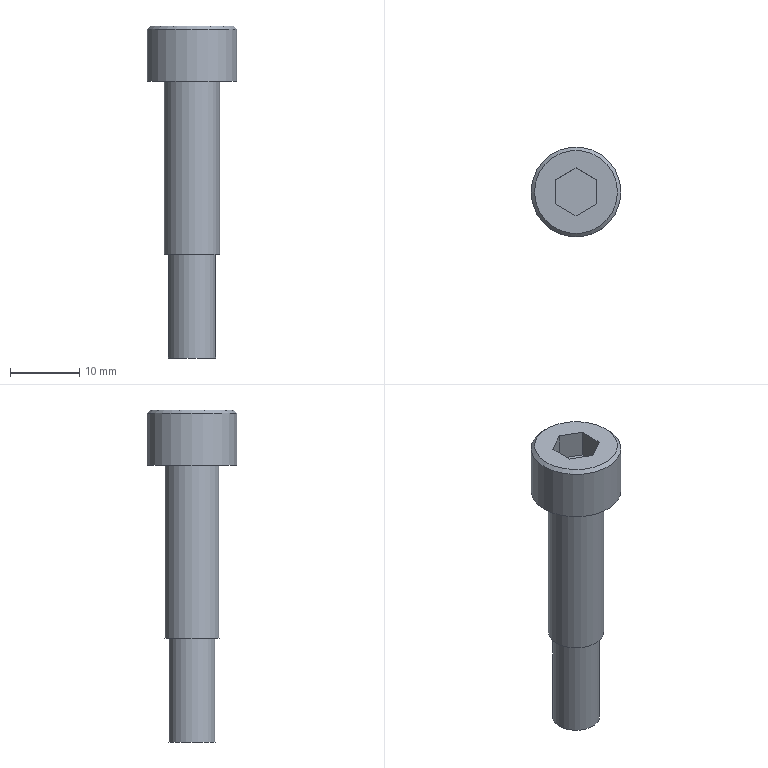Part | STEP file | M3-10_id154_x_t | 1 solid | 15 faces | box 13 x 13 x 48 mm | volume 2734 mm3 | plane 11 | cylinder 3 | cone 1 | commonest cylinder face diameters 6.8 x1 8 x1 13 x1
STEP:
#1=CARTESIAN_POINT('',(-180.986,-124.,-47.));
#2=VERTEX_POINT('',#1);
#3=CARTESIAN_POINT('',(-177.586,-124.,-47.));
#4=DIRECTION('',(0.,0.,-1.));
#5=DIRECTION('',(-1.,0.,0.));
#6=AXIS2_PLACEMENT_3D('',#3,#4,#5);
#7=CIRCLE('',#6,3.4);
#8=EDGE_CURVE('',#2,#2,#7,.T.);
#9=ORIENTED_EDGE('',*,*,#8,.F.);
#10=EDGE_LOOP('',(#9));
#11=FACE_BOUND('',#10,.T.);
#12=CARTESIAN_POINT('',(-173.586,-124.,-47.));
#13=VERTEX_POINT('',#12);
#14=CARTESIAN_POINT('',(-177.586,-124.,-47.));
#15=DIRECTION('',(0.,0.,1.));
#16=DIRECTION('',(1.,0.,0.));
#17=AXIS2_PLACEMENT_3D('',#14,#15,#16);
#18=CIRCLE('',#17,4.);
#19=EDGE_CURVE('',#13,#13,#18,.T.);
#20=ORIENTED_EDGE('',*,*,#19,.F.);
#21=EDGE_LOOP('',(#20));
#22=FACE_BOUND('',#21,.T.);
#23=CARTESIAN_POINT('',(-177.586,-124.,-47.));
#24=DIRECTION('',(0.,0.,-1.));
#25=DIRECTION('',(-1.,0.,0.));
#26=AXIS2_PLACEMENT_3D('',#23,#24,#25);
#27=PLANE('',#26);
#28=ADVANCED_FACE('',(#11,#22),#27,.T.);
#29=CARTESIAN_POINT('',(-181.586,-124.,-22.));
#30=VERTEX_POINT('',#29);
#31=CARTESIAN_POINT('',(-177.586,-124.,-22.));
#32=DIRECTION('',(0.,0.,1.));
#33=DIRECTION('',(-1.,0.,0.));
#34=AXIS2_PLACEMENT_3D('',#31,#32,#33);
#35=CIRCLE('',#34,4.);
#36=EDGE_CURVE('',#30,#30,#35,.T.);
#37=ORIENTED_EDGE('',*,*,#36,.F.);
#38=EDGE_LOOP('',(#37));
#39=FACE_BOUND('',#38,.T.);
#40=ORIENTED_EDGE('',*,*,#19,.T.);
#41=EDGE_LOOP('',(#40));
#42=FACE_BOUND('',#41,.T.);
#43=CARTESIAN_POINT('',(-177.586,-124.,-47.));
#44=DIRECTION('',(0.,0.,1.));
#45=DIRECTION('',(1.,0.,0.));
#46=AXIS2_PLACEMENT_3D('',#43,#44,#45);
#47=CYLINDRICAL_SURFACE('',#46,4.);
#48=ADVANCED_FACE('',(#39,#42),#47,.T.);
#49=CARTESIAN_POINT('',(-174.186,-124.,-62.));
#50=VERTEX_POINT('',#49);
#51=CARTESIAN_POINT('',(-177.586,-124.,-62.));
#52=DIRECTION('',(0.,0.,1.));
#53=DIRECTION('',(1.,0.,0.));
#54=AXIS2_PLACEMENT_3D('',#51,#52,#53);
#55=CIRCLE('',#54,3.4);
#56=EDGE_CURVE('',#50,#50,#55,.T.);
#57=ORIENTED_EDGE('',*,*,#56,.F.);
#58=EDGE_LOOP('',(#57));
#59=FACE_OUTER_BOUND('',#58,.T.);
#60=CARTESIAN_POINT('',(-177.586,-124.,-62.));
#61=DIRECTION('',(0.,0.,-1.));
#62=DIRECTION('',(-1.,0.,0.));
#63=AXIS2_PLACEMENT_3D('',#60,#61,#62);
#64=PLANE('',#63);
#65=ADVANCED_FACE('',(#59),#64,.T.);
#66=ORIENTED_EDGE('',*,*,#56,.T.);
#67=EDGE_LOOP('',(#66));
#68=FACE_BOUND('',#67,.T.);
#69=ORIENTED_EDGE('',*,*,#8,.T.);
#70=EDGE_LOOP('',(#69));
#71=FACE_BOUND('',#70,.T.);
#72=CARTESIAN_POINT('',(-177.586,-124.,-47.));
#73=DIRECTION('',(0.,0.,-1.));
#74=DIRECTION('',(1.,0.,0.));
#75=AXIS2_PLACEMENT_3D('',#72,#73,#74);
#76=CYLINDRICAL_SURFACE('',#75,3.4);
#77=ADVANCED_FACE('',(#68,#71),#76,.T.);
#78=CARTESIAN_POINT('',(-180.586,-122.268,-14.));
#79=VERTEX_POINT('',#78);
#80=CARTESIAN_POINT('',(-180.586,-125.732,-14.));
#81=VERTEX_POINT('',#80);
#82=CARTESIAN_POINT('',(-180.586,-122.268,-14.));
#83=DIRECTION('',(0.,-1.,0.));
#84=VECTOR('',#83,1.);
#85=LINE('',#82,#84);
#86=EDGE_CURVE('',#79,#81,#85,.T.);
#87=ORIENTED_EDGE('',*,*,#86,.F.);
#88=CARTESIAN_POINT('',(-177.586,-120.536,-14.));
#89=VERTEX_POINT('',#88);
#90=CARTESIAN_POINT('',(-177.586,-120.536,-14.));
#91=DIRECTION('',(-0.866,-0.5,0.));
#92=VECTOR('',#91,1.);
#93=LINE('',#90,#92);
#94=EDGE_CURVE('',#89,#79,#93,.T.);
#95=ORIENTED_EDGE('',*,*,#94,.F.);
#96=CARTESIAN_POINT('',(-174.586,-122.268,-14.));
#97=VERTEX_POINT('',#96);
#98=CARTESIAN_POINT('',(-174.586,-122.268,-14.));
#99=DIRECTION('',(-0.866,0.5,0.));
#100=VECTOR('',#99,1.);
#101=LINE('',#98,#100);
#102=EDGE_CURVE('',#97,#89,#101,.T.);
#103=ORIENTED_EDGE('',*,*,#102,.F.);
#104=CARTESIAN_POINT('',(-174.586,-125.732,-14.));
#105=VERTEX_POINT('',#104);
#106=CARTESIAN_POINT('',(-174.586,-125.732,-14.));
#107=DIRECTION('',(0.,1.,0.));
#108=VECTOR('',#107,1.);
#109=LINE('',#106,#108);
#110=EDGE_CURVE('',#105,#97,#109,.T.);
#111=ORIENTED_EDGE('',*,*,#110,.F.);
#112=CARTESIAN_POINT('',(-177.586,-127.464,-14.));
#113=VERTEX_POINT('',#112);
#114=CARTESIAN_POINT('',(-177.586,-127.464,-14.));
#115=DIRECTION('',(0.866,0.5,0.));
#116=VECTOR('',#115,1.);
#117=LINE('',#114,#116);
#118=EDGE_CURVE('',#113,#105,#117,.T.);
#119=ORIENTED_EDGE('',*,*,#118,.F.);
#120=CARTESIAN_POINT('',(-180.586,-125.732,-14.));
#121=DIRECTION('',(0.866,-0.5,0.));
#122=VECTOR('',#121,1.);
#123=LINE('',#120,#122);
#124=EDGE_CURVE('',#81,#113,#123,.T.);
#125=ORIENTED_EDGE('',*,*,#124,.F.);
#126=EDGE_LOOP('',(#87,#95,#103,#111,#119,#125));
#127=FACE_BOUND('',#126,.T.);
#128=CARTESIAN_POINT('',(-171.586,-124.,-14.));
#129=VERTEX_POINT('',#128);
#130=CARTESIAN_POINT('',(-177.586,-124.,-14.));
#131=DIRECTION('',(0.,0.,1.));
#132=DIRECTION('',(1.,0.,0.));
#133=AXIS2_PLACEMENT_3D('',#130,#131,#132);
#134=CIRCLE('',#133,6.);
#135=EDGE_CURVE('',#129,#129,#134,.T.);
#136=ORIENTED_EDGE('',*,*,#135,.T.);
#137=EDGE_LOOP('',(#136));
#138=FACE_BOUND('',#137,.T.);
#139=CARTESIAN_POINT('',(-177.586,-124.,-14.));
#140=DIRECTION('',(0.,0.,1.));
#141=DIRECTION('',(1.,0.,0.));
#142=AXIS2_PLACEMENT_3D('',#139,#140,#141);
#143=PLANE('',#142);
#144=ADVANCED_FACE('',(#127,#138),#143,.T.);
#145=ORIENTED_EDGE('',*,*,#36,.T.);
#146=EDGE_LOOP('',(#145));
#147=FACE_BOUND('',#146,.T.);
#148=CARTESIAN_POINT('',(-171.086,-124.,-22.));
#149=VERTEX_POINT('',#148);
#150=CARTESIAN_POINT('',(-177.586,-124.,-22.));
#151=DIRECTION('',(0.,0.,1.));
#152=DIRECTION('',(1.,0.,0.));
#153=AXIS2_PLACEMENT_3D('',#150,#151,#152);
#154=CIRCLE('',#153,6.5);
#155=EDGE_CURVE('',#149,#149,#154,.T.);
#156=ORIENTED_EDGE('',*,*,#155,.F.);
#157=EDGE_LOOP('',(#156));
#158=FACE_BOUND('',#157,.T.);
#159=CARTESIAN_POINT('',(-177.586,-124.,-22.));
#160=DIRECTION('',(0.,0.,-1.));
#161=DIRECTION('',(-1.,0.,0.));
#162=AXIS2_PLACEMENT_3D('',#159,#160,#161);
#163=PLANE('',#162);
#164=ADVANCED_FACE('',(#147,#158),#163,.T.);
#165=CARTESIAN_POINT('',(-171.086,-124.,-14.5));
#166=VERTEX_POINT('',#165);
#167=CARTESIAN_POINT('',(-177.586,-124.,-14.5));
#168=DIRECTION('',(0.,0.,-1.));
#169=DIRECTION('',(1.,0.,0.));
#170=AXIS2_PLACEMENT_3D('',#167,#168,#169);
#171=CIRCLE('',#170,6.5);
#172=EDGE_CURVE('',#166,#166,#171,.T.);
#173=ORIENTED_EDGE('',*,*,#172,.T.);
#174=EDGE_LOOP('',(#173));
#175=FACE_BOUND('',#174,.T.);
#176=ORIENTED_EDGE('',*,*,#155,.T.);
#177=EDGE_LOOP('',(#176));
#178=FACE_BOUND('',#177,.T.);
#179=CARTESIAN_POINT('',(-177.586,-124.,-22.));
#180=DIRECTION('',(0.,0.,1.));
#181=DIRECTION('',(1.,0.,0.));
#182=AXIS2_PLACEMENT_3D('',#179,#180,#181);
#183=CYLINDRICAL_SURFACE('',#182,6.5);
#184=ADVANCED_FACE('',(#175,#178),#183,.T.);
#185=ORIENTED_EDGE('',*,*,#135,.F.);
#186=EDGE_LOOP('',(#185));
#187=FACE_BOUND('',#186,.T.);
#188=ORIENTED_EDGE('',*,*,#172,.F.);
#189=EDGE_LOOP('',(#188));
#190=FACE_BOUND('',#189,.T.);
#191=CARTESIAN_POINT('',(-177.586,-124.,-14.5));
#192=DIRECTION('',(0.,0.,-1.));
#193=DIRECTION('',(-1.,0.,0.));
#194=AXIS2_PLACEMENT_3D('',#191,#192,#193);
#195=CONICAL_SURFACE('',#194,6.5,45.);
#196=ADVANCED_FACE('',(#187,#190),#195,.T.);
#197=ORIENTED_EDGE('',*,*,#86,.T.);
#198=CARTESIAN_POINT('',(-180.586,-125.732,-18.));
#199=VERTEX_POINT('',#198);
#200=CARTESIAN_POINT('',(-180.586,-125.732,-18.));
#201=DIRECTION('',(0.,0.,-1.));
#202=VECTOR('',#201,1.);
#203=LINE('',#200,#202);
#204=EDGE_CURVE('',#81,#199,#203,.T.);
#205=ORIENTED_EDGE('',*,*,#204,.T.);
#206=CARTESIAN_POINT('',(-180.586,-122.268,-18.));
#207=VERTEX_POINT('',#206);
#208=CARTESIAN_POINT('',(-180.586,-122.268,-18.));
#209=DIRECTION('',(0.,1.,0.));
#210=VECTOR('',#209,1.);
#211=LINE('',#208,#210);
#212=EDGE_CURVE('',#199,#207,#211,.T.);
#213=ORIENTED_EDGE('',*,*,#212,.T.);
#214=CARTESIAN_POINT('',(-180.586,-122.268,-18.));
#215=DIRECTION('',(0.,0.,-1.));
#216=VECTOR('',#215,1.);
#217=LINE('',#214,#216);
#218=EDGE_CURVE('',#79,#207,#217,.T.);
#219=ORIENTED_EDGE('',*,*,#218,.F.);
#220=EDGE_LOOP('',(#197,#205,#213,#219));
#221=FACE_OUTER_BOUND('',#220,.T.);
#222=CARTESIAN_POINT('',(-180.586,-122.268,-18.));
#223=DIRECTION('',(-1.,0.,0.));
#224=DIRECTION('',(0.,-1.,0.));
#225=AXIS2_PLACEMENT_3D('',#222,#223,#224);
#226=PLANE('',#225);
#227=ADVANCED_FACE('',(#221),#226,.F.);
#228=ORIENTED_EDGE('',*,*,#124,.T.);
#229=CARTESIAN_POINT('',(-177.586,-127.464,-18.));
#230=VERTEX_POINT('',#229);
#231=CARTESIAN_POINT('',(-177.586,-127.464,-18.));
#232=DIRECTION('',(0.,0.,-1.));
#233=VECTOR('',#232,1.);
#234=LINE('',#231,#233);
#235=EDGE_CURVE('',#113,#230,#234,.T.);
#236=ORIENTED_EDGE('',*,*,#235,.T.);
#237=CARTESIAN_POINT('',(-180.586,-125.732,-18.));
#238=DIRECTION('',(-0.866,0.5,0.));
#239=VECTOR('',#238,1.);
#240=LINE('',#237,#239);
#241=EDGE_CURVE('',#230,#199,#240,.T.);
#242=ORIENTED_EDGE('',*,*,#241,.T.);
#243=ORIENTED_EDGE('',*,*,#204,.F.);
#244=EDGE_LOOP('',(#228,#236,#242,#243));
#245=FACE_OUTER_BOUND('',#244,.T.);
#246=CARTESIAN_POINT('',(-180.586,-125.732,-18.));
#247=DIRECTION('',(-0.5,-0.866,0.));
#248=DIRECTION('',(0.866,-0.5,0.));
#249=AXIS2_PLACEMENT_3D('',#246,#247,#248);
#250=PLANE('',#249);
#251=ADVANCED_FACE('',(#245),#250,.F.);
#252=ORIENTED_EDGE('',*,*,#118,.T.);
#253=CARTESIAN_POINT('',(-174.586,-125.732,-18.));
#254=VERTEX_POINT('',#253);
#255=CARTESIAN_POINT('',(-174.586,-125.732,-18.));
#256=DIRECTION('',(0.,0.,-1.));
#257=VECTOR('',#256,1.);
#258=LINE('',#255,#257);
#259=EDGE_CURVE('',#105,#254,#258,.T.);
#260=ORIENTED_EDGE('',*,*,#259,.T.);
#261=CARTESIAN_POINT('',(-177.586,-127.464,-18.));
#262=DIRECTION('',(-0.866,-0.5,0.));
#263=VECTOR('',#262,1.);
#264=LINE('',#261,#263);
#265=EDGE_CURVE('',#254,#230,#264,.T.);
#266=ORIENTED_EDGE('',*,*,#265,.T.);
#267=ORIENTED_EDGE('',*,*,#235,.F.);
#268=EDGE_LOOP('',(#252,#260,#266,#267));
#269=FACE_OUTER_BOUND('',#268,.T.);
#270=CARTESIAN_POINT('',(-177.586,-127.464,-18.));
#271=DIRECTION('',(0.5,-0.866,0.));
#272=DIRECTION('',(0.866,0.5,0.));
#273=AXIS2_PLACEMENT_3D('',#270,#271,#272);
#274=PLANE('',#273);
#275=ADVANCED_FACE('',(#269),#274,.F.);
#276=ORIENTED_EDGE('',*,*,#110,.T.);
#277=CARTESIAN_POINT('',(-174.586,-122.268,-18.));
#278=VERTEX_POINT('',#277);
#279=CARTESIAN_POINT('',(-174.586,-122.268,-18.));
#280=DIRECTION('',(0.,0.,-1.));
#281=VECTOR('',#280,1.);
#282=LINE('',#279,#281);
#283=EDGE_CURVE('',#97,#278,#282,.T.);
#284=ORIENTED_EDGE('',*,*,#283,.T.);
#285=CARTESIAN_POINT('',(-174.586,-125.732,-18.));
#286=DIRECTION('',(0.,-1.,0.));
#287=VECTOR('',#286,1.);
#288=LINE('',#285,#287);
#289=EDGE_CURVE('',#278,#254,#288,.T.);
#290=ORIENTED_EDGE('',*,*,#289,.T.);
#291=ORIENTED_EDGE('',*,*,#259,.F.);
#292=EDGE_LOOP('',(#276,#284,#290,#291));
#293=FACE_OUTER_BOUND('',#292,.T.);
#294=CARTESIAN_POINT('',(-174.586,-125.732,-18.));
#295=DIRECTION('',(1.,0.,0.));
#296=DIRECTION('',(0.,1.,0.));
#297=AXIS2_PLACEMENT_3D('',#294,#295,#296);
#298=PLANE('',#297);
#299=ADVANCED_FACE('',(#293),#298,.F.);
#300=ORIENTED_EDGE('',*,*,#102,.T.);
#301=CARTESIAN_POINT('',(-177.586,-120.536,-18.));
#302=VERTEX_POINT('',#301);
#303=CARTESIAN_POINT('',(-177.586,-120.536,-18.));
#304=DIRECTION('',(0.,0.,-1.));
#305=VECTOR('',#304,1.);
#306=LINE('',#303,#305);
#307=EDGE_CURVE('',#89,#302,#306,.T.);
#308=ORIENTED_EDGE('',*,*,#307,.T.);
#309=CARTESIAN_POINT('',(-174.586,-122.268,-18.));
#310=DIRECTION('',(0.866,-0.5,0.));
#311=VECTOR('',#310,1.);
#312=LINE('',#309,#311);
#313=EDGE_CURVE('',#302,#278,#312,.T.);
#314=ORIENTED_EDGE('',*,*,#313,.T.);
#315=ORIENTED_EDGE('',*,*,#283,.F.);
#316=EDGE_LOOP('',(#300,#308,#314,#315));
#317=FACE_OUTER_BOUND('',#316,.T.);
#318=CARTESIAN_POINT('',(-174.586,-122.268,-18.));
#319=DIRECTION('',(0.5,0.866,0.));
#320=DIRECTION('',(-0.866,0.5,0.));
#321=AXIS2_PLACEMENT_3D('',#318,#319,#320);
#322=PLANE('',#321);
#323=ADVANCED_FACE('',(#317),#322,.F.);
#324=ORIENTED_EDGE('',*,*,#94,.T.);
#325=ORIENTED_EDGE('',*,*,#218,.T.);
#326=CARTESIAN_POINT('',(-177.586,-120.536,-18.));
#327=DIRECTION('',(0.866,0.5,0.));
#328=VECTOR('',#327,1.);
#329=LINE('',#326,#328);
#330=EDGE_CURVE('',#207,#302,#329,.T.);
#331=ORIENTED_EDGE('',*,*,#330,.T.);
#332=ORIENTED_EDGE('',*,*,#307,.F.);
#333=EDGE_LOOP('',(#324,#325,#331,#332));
#334=FACE_OUTER_BOUND('',#333,.T.);
#335=CARTESIAN_POINT('',(-177.586,-120.536,-18.));
#336=DIRECTION('',(-0.5,0.866,0.));
#337=DIRECTION('',(-0.866,-0.5,0.));
#338=AXIS2_PLACEMENT_3D('',#335,#336,#337);
#339=PLANE('',#338);
#340=ADVANCED_FACE('',(#334),#339,.F.);
#341=ORIENTED_EDGE('',*,*,#212,.F.);
#342=ORIENTED_EDGE('',*,*,#241,.F.);
#343=ORIENTED_EDGE('',*,*,#265,.F.);
#344=ORIENTED_EDGE('',*,*,#289,.F.);
#345=ORIENTED_EDGE('',*,*,#313,.F.);
#346=ORIENTED_EDGE('',*,*,#330,.F.);
#347=EDGE_LOOP('',(#341,#342,#343,#344,#345,#346));
#348=FACE_OUTER_BOUND('',#347,.T.);
#349=CARTESIAN_POINT('',(-177.586,-124.,-18.));
#350=DIRECTION('',(0.,0.,1.));
#351=DIRECTION('',(1.,0.,0.));
#352=AXIS2_PLACEMENT_3D('',#349,#350,#351);
#353=PLANE('',#352);
#354=ADVANCED_FACE('',(#348),#353,.T.);
#355=CLOSED_SHELL('',(#28,#48,#65,#77,#144,#164,#184,#196,#227,#251,#275,#299,#323,#340,#354));
#356=MANIFOLD_SOLID_BREP('',#355);
#357=(LENGTH_UNIT()NAMED_UNIT(*)SI_UNIT(.MILLI.,.METRE.));
#358=UNCERTAINTY_MEASURE_WITH_UNIT(LENGTH_MEASURE(0.00002),#357,'','');
#359=(NAMED_UNIT(*)PLANE_ANGLE_UNIT()SI_UNIT($,.RADIAN.));
#360=PLANE_ANGLE_MEASURE_WITH_UNIT(PLANE_ANGLE_MEASURE(0.01745),#359);
#361=DIMENSIONAL_EXPONENTS(0.,0.,0.,0.,0.,0.,0.);
#362=(CONVERSION_BASED_UNIT('DEGREE',#360)NAMED_UNIT(#361)PLANE_ANGLE_UNIT());
#363=(NAMED_UNIT(*)SI_UNIT($,.STERADIAN.)SOLID_ANGLE_UNIT());
#364=(GEOMETRIC_REPRESENTATION_CONTEXT(3)GLOBAL_UNCERTAINTY_ASSIGNED_CONTEXT((#358))GLOBAL_UNIT_ASSIGNED_CONTEXT((#357,#362,#363))REPRESENTATION_CONTEXT('',''));
#365=ADVANCED_BREP_SHAPE_REPRESENTATION('',(#356),#364);